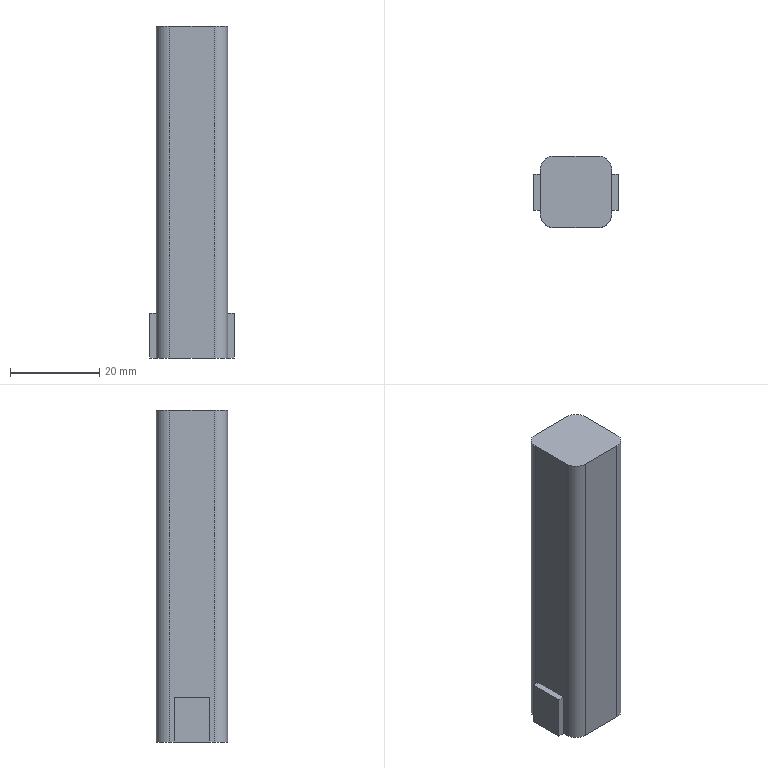Part | NX | features solid 2 | 1 solid | 18 faces | box 19 x 16 x 74.5 mm | volume 18736 mm3 | plane 14 | cylinder 4 | commonest cylinder face diameters 6 x4
STEP:
#1=CARTESIAN_POINT('',(2052.,45.,-68.));
#2=VERTEX_POINT('',#1);
#3=CARTESIAN_POINT('',(2052.,37.,-68.));
#4=VERTEX_POINT('',#3);
#5=CARTESIAN_POINT('',(2052.,41.,-68.));
#6=DIRECTION('',(0.,-1.,0.));
#7=VECTOR('',#6,1000.);
#8=LINE('',#5,#7);
#9=EDGE_CURVE('',#2,#4,#8,.T.);
#10=ORIENTED_EDGE('',*,*,#9,.T.);
#11=CARTESIAN_POINT('',(2052.,37.,-78.));
#12=VERTEX_POINT('',#11);
#13=CARTESIAN_POINT('',(2052.,37.,-63.));
#14=DIRECTION('',(0.,0.,-1.));
#15=VECTOR('',#14,1000.);
#16=LINE('',#13,#15);
#17=EDGE_CURVE('',#4,#12,#16,.T.);
#18=ORIENTED_EDGE('',*,*,#17,.T.);
#19=CARTESIAN_POINT('',(2052.,36.,-78.));
#20=VERTEX_POINT('',#19);
#21=CARTESIAN_POINT('',(2052.,41.,-78.));
#22=DIRECTION('',(0.,1.,0.));
#23=VECTOR('',#22,1000.);
#24=LINE('',#21,#23);
#25=EDGE_CURVE('',#20,#12,#24,.T.);
#26=ORIENTED_EDGE('',*,*,#25,.F.);
#27=CARTESIAN_POINT('',(2052.,36.,-3.5));
#28=VERTEX_POINT('',#27);
#29=CARTESIAN_POINT('',(2052.,36.,-63.));
#30=DIRECTION('',(0.,0.,1.));
#31=VECTOR('',#30,1000.);
#32=LINE('',#29,#31);
#33=EDGE_CURVE('',#20,#28,#32,.T.);
#34=ORIENTED_EDGE('',*,*,#33,.T.);
#35=CARTESIAN_POINT('',(2052.,46.,-3.5));
#36=VERTEX_POINT('',#35);
#37=CARTESIAN_POINT('',(2052.,41.,-3.5));
#38=DIRECTION('',(0.,1.,0.));
#39=VECTOR('',#38,1000.);
#40=LINE('',#37,#39);
#41=EDGE_CURVE('',#28,#36,#40,.T.);
#42=ORIENTED_EDGE('',*,*,#41,.T.);
#43=CARTESIAN_POINT('',(2052.,46.,-78.));
#44=VERTEX_POINT('',#43);
#45=CARTESIAN_POINT('',(2052.,46.,-63.));
#46=DIRECTION('',(0.,0.,-1.));
#47=VECTOR('',#46,1000.);
#48=LINE('',#45,#47);
#49=EDGE_CURVE('',#36,#44,#48,.T.);
#50=ORIENTED_EDGE('',*,*,#49,.T.);
#51=CARTESIAN_POINT('',(2052.,45.,-78.));
#52=VERTEX_POINT('',#51);
#53=CARTESIAN_POINT('',(2052.,41.,-78.));
#54=DIRECTION('',(0.,1.,0.));
#55=VECTOR('',#54,1000.);
#56=LINE('',#53,#55);
#57=EDGE_CURVE('',#52,#44,#56,.T.);
#58=ORIENTED_EDGE('',*,*,#57,.F.);
#59=CARTESIAN_POINT('',(2052.,45.,-63.));
#60=DIRECTION('',(0.,0.,1.));
#61=VECTOR('',#60,1000.);
#62=LINE('',#59,#61);
#63=EDGE_CURVE('',#52,#2,#62,.T.);
#64=ORIENTED_EDGE('',*,*,#63,.T.);
#65=EDGE_LOOP('',(#10,#18,#26,#34,#42,#50,#58,#64));
#66=FACE_BOUND('',#65,.T.);
#67=CARTESIAN_POINT('',(2052.,41.,-63.));
#68=DIRECTION('',(-1.,0.,0.));
#69=DIRECTION('',(0.,0.,-1.));
#70=AXIS2_PLACEMENT_3D('',#67,#68,#69);
#71=PLANE('',#70);
#72=ADVANCED_FACE('',(#66),#71,.T.);
#73=ORIENTED_EDGE('',*,*,#41,.F.);
#74=CARTESIAN_POINT('',(2055.,33.,-3.5));
#75=VERTEX_POINT('',#74);
#76=CARTESIAN_POINT('',(2055.,36.,-3.5));
#77=DIRECTION('',(0.,0.,1.));
#78=DIRECTION('',(1.,0.,0.));
#79=AXIS2_PLACEMENT_3D('',#76,#77,#78);
#80=CIRCLE('',#79,3.);
#81=EDGE_CURVE('',#28,#75,#80,.T.);
#82=ORIENTED_EDGE('',*,*,#81,.T.);
#83=CARTESIAN_POINT('',(2065.,33.,-3.5));
#84=VERTEX_POINT('',#83);
#85=CARTESIAN_POINT('',(2060.,33.,-3.5));
#86=DIRECTION('',(-1.,0.,0.));
#87=VECTOR('',#86,1000.);
#88=LINE('',#85,#87);
#89=EDGE_CURVE('',#84,#75,#88,.T.);
#90=ORIENTED_EDGE('',*,*,#89,.F.);
#91=CARTESIAN_POINT('',(2068.,36.,-3.5));
#92=VERTEX_POINT('',#91);
#93=CARTESIAN_POINT('',(2065.,36.,-3.5));
#94=DIRECTION('',(0.,0.,1.));
#95=DIRECTION('',(1.,0.,0.));
#96=AXIS2_PLACEMENT_3D('',#93,#94,#95);
#97=CIRCLE('',#96,3.);
#98=EDGE_CURVE('',#84,#92,#97,.T.);
#99=ORIENTED_EDGE('',*,*,#98,.T.);
#100=CARTESIAN_POINT('',(2068.,46.,-3.5));
#101=VERTEX_POINT('',#100);
#102=CARTESIAN_POINT('',(2068.,41.,-3.5));
#103=DIRECTION('',(0.,-1.,0.));
#104=VECTOR('',#103,1000.);
#105=LINE('',#102,#104);
#106=EDGE_CURVE('',#101,#92,#105,.T.);
#107=ORIENTED_EDGE('',*,*,#106,.F.);
#108=CARTESIAN_POINT('',(2065.,49.,-3.5));
#109=VERTEX_POINT('',#108);
#110=CARTESIAN_POINT('',(2065.,46.,-3.5));
#111=DIRECTION('',(0.,0.,1.));
#112=DIRECTION('',(1.,0.,0.));
#113=AXIS2_PLACEMENT_3D('',#110,#111,#112);
#114=CIRCLE('',#113,3.);
#115=EDGE_CURVE('',#101,#109,#114,.T.);
#116=ORIENTED_EDGE('',*,*,#115,.T.);
#117=CARTESIAN_POINT('',(2055.,49.,-3.5));
#118=VERTEX_POINT('',#117);
#119=CARTESIAN_POINT('',(2060.,49.,-3.5));
#120=DIRECTION('',(1.,0.,0.));
#121=VECTOR('',#120,1000.);
#122=LINE('',#119,#121);
#123=EDGE_CURVE('',#118,#109,#122,.T.);
#124=ORIENTED_EDGE('',*,*,#123,.F.);
#125=CARTESIAN_POINT('',(2055.,46.,-3.5));
#126=DIRECTION('',(0.,0.,1.));
#127=DIRECTION('',(1.,0.,0.));
#128=AXIS2_PLACEMENT_3D('',#125,#126,#127);
#129=CIRCLE('',#128,3.);
#130=EDGE_CURVE('',#118,#36,#129,.T.);
#131=ORIENTED_EDGE('',*,*,#130,.T.);
#132=EDGE_LOOP('',(#73,#82,#90,#99,#107,#116,#124,#131));
#133=FACE_BOUND('',#132,.T.);
#134=CARTESIAN_POINT('',(2060.,41.,-3.5));
#135=DIRECTION('',(0.,0.,1.));
#136=DIRECTION('',(-1.,0.,0.));
#137=AXIS2_PLACEMENT_3D('',#134,#135,#136);
#138=PLANE('',#137);
#139=ADVANCED_FACE('',(#133),#138,.T.);
#140=CARTESIAN_POINT('',(2055.,33.,-78.));
#141=VERTEX_POINT('',#140);
#142=CARTESIAN_POINT('',(2065.,33.,-78.));
#143=VERTEX_POINT('',#142);
#144=CARTESIAN_POINT('',(2060.,33.,-78.));
#145=DIRECTION('',(1.,0.,0.));
#146=VECTOR('',#145,1000.);
#147=LINE('',#144,#146);
#148=EDGE_CURVE('',#141,#143,#147,.T.);
#149=ORIENTED_EDGE('',*,*,#148,.T.);
#150=CARTESIAN_POINT('',(2065.,33.,-63.));
#151=DIRECTION('',(0.,0.,1.));
#152=VECTOR('',#151,1000.);
#153=LINE('',#150,#152);
#154=EDGE_CURVE('',#143,#84,#153,.T.);
#155=ORIENTED_EDGE('',*,*,#154,.T.);
#156=ORIENTED_EDGE('',*,*,#89,.T.);
#157=CARTESIAN_POINT('',(2055.,33.,-63.));
#158=DIRECTION('',(0.,0.,-1.));
#159=VECTOR('',#158,1000.);
#160=LINE('',#157,#159);
#161=EDGE_CURVE('',#75,#141,#160,.T.);
#162=ORIENTED_EDGE('',*,*,#161,.T.);
#163=EDGE_LOOP('',(#149,#155,#156,#162));
#164=FACE_BOUND('',#163,.T.);
#165=CARTESIAN_POINT('',(2060.,33.,-63.));
#166=DIRECTION('',(0.,-1.,0.));
#167=DIRECTION('',(0.,0.,1.));
#168=AXIS2_PLACEMENT_3D('',#165,#166,#167);
#169=PLANE('',#168);
#170=ADVANCED_FACE('',(#164),#169,.T.);
#171=CARTESIAN_POINT('',(2065.,49.,-78.));
#172=VERTEX_POINT('',#171);
#173=CARTESIAN_POINT('',(2055.,49.,-78.));
#174=VERTEX_POINT('',#173);
#175=CARTESIAN_POINT('',(2060.,49.,-78.));
#176=DIRECTION('',(-1.,0.,0.));
#177=VECTOR('',#176,1000.);
#178=LINE('',#175,#177);
#179=EDGE_CURVE('',#172,#174,#178,.T.);
#180=ORIENTED_EDGE('',*,*,#179,.T.);
#181=CARTESIAN_POINT('',(2055.,49.,-63.));
#182=DIRECTION('',(0.,0.,1.));
#183=VECTOR('',#182,1000.);
#184=LINE('',#181,#183);
#185=EDGE_CURVE('',#174,#118,#184,.T.);
#186=ORIENTED_EDGE('',*,*,#185,.T.);
#187=ORIENTED_EDGE('',*,*,#123,.T.);
#188=CARTESIAN_POINT('',(2065.,49.,-63.));
#189=DIRECTION('',(0.,0.,-1.));
#190=VECTOR('',#189,1000.);
#191=LINE('',#188,#190);
#192=EDGE_CURVE('',#109,#172,#191,.T.);
#193=ORIENTED_EDGE('',*,*,#192,.T.);
#194=EDGE_LOOP('',(#180,#186,#187,#193));
#195=FACE_BOUND('',#194,.T.);
#196=CARTESIAN_POINT('',(2060.,49.,-63.));
#197=DIRECTION('',(0.,1.,0.));
#198=DIRECTION('',(0.,0.,-1.));
#199=AXIS2_PLACEMENT_3D('',#196,#197,#198);
#200=PLANE('',#199);
#201=ADVANCED_FACE('',(#195),#200,.T.);
#202=CARTESIAN_POINT('',(2068.,45.,-78.));
#203=VERTEX_POINT('',#202);
#204=CARTESIAN_POINT('',(2068.,45.,-68.));
#205=VERTEX_POINT('',#204);
#206=CARTESIAN_POINT('',(2068.,45.,-63.));
#207=DIRECTION('',(0.,0.,1.));
#208=VECTOR('',#207,1000.);
#209=LINE('',#206,#208);
#210=EDGE_CURVE('',#203,#205,#209,.T.);
#211=ORIENTED_EDGE('',*,*,#210,.F.);
#212=CARTESIAN_POINT('',(2068.,46.,-78.));
#213=VERTEX_POINT('',#212);
#214=CARTESIAN_POINT('',(2068.,41.,-78.));
#215=DIRECTION('',(0.,-1.,0.));
#216=VECTOR('',#215,1000.);
#217=LINE('',#214,#216);
#218=EDGE_CURVE('',#213,#203,#217,.T.);
#219=ORIENTED_EDGE('',*,*,#218,.F.);
#220=CARTESIAN_POINT('',(2068.,46.,-63.));
#221=DIRECTION('',(0.,0.,1.));
#222=VECTOR('',#221,1000.);
#223=LINE('',#220,#222);
#224=EDGE_CURVE('',#213,#101,#223,.T.);
#225=ORIENTED_EDGE('',*,*,#224,.T.);
#226=ORIENTED_EDGE('',*,*,#106,.T.);
#227=CARTESIAN_POINT('',(2068.,36.,-78.));
#228=VERTEX_POINT('',#227);
#229=CARTESIAN_POINT('',(2068.,36.,-63.));
#230=DIRECTION('',(0.,0.,-1.));
#231=VECTOR('',#230,1000.);
#232=LINE('',#229,#231);
#233=EDGE_CURVE('',#92,#228,#232,.T.);
#234=ORIENTED_EDGE('',*,*,#233,.T.);
#235=CARTESIAN_POINT('',(2068.,37.,-78.));
#236=VERTEX_POINT('',#235);
#237=CARTESIAN_POINT('',(2068.,41.,-78.));
#238=DIRECTION('',(0.,-1.,0.));
#239=VECTOR('',#238,1000.);
#240=LINE('',#237,#239);
#241=EDGE_CURVE('',#236,#228,#240,.T.);
#242=ORIENTED_EDGE('',*,*,#241,.F.);
#243=CARTESIAN_POINT('',(2068.,37.,-68.));
#244=VERTEX_POINT('',#243);
#245=CARTESIAN_POINT('',(2068.,37.,-63.));
#246=DIRECTION('',(0.,0.,-1.));
#247=VECTOR('',#246,1000.);
#248=LINE('',#245,#247);
#249=EDGE_CURVE('',#244,#236,#248,.T.);
#250=ORIENTED_EDGE('',*,*,#249,.F.);
#251=CARTESIAN_POINT('',(2068.,41.,-68.));
#252=DIRECTION('',(0.,-1.,0.));
#253=VECTOR('',#252,1000.);
#254=LINE('',#251,#253);
#255=EDGE_CURVE('',#205,#244,#254,.T.);
#256=ORIENTED_EDGE('',*,*,#255,.F.);
#257=EDGE_LOOP('',(#211,#219,#225,#226,#234,#242,#250,#256));
#258=FACE_BOUND('',#257,.T.);
#259=CARTESIAN_POINT('',(2068.,41.,-63.));
#260=DIRECTION('',(1.,0.,0.));
#261=DIRECTION('',(0.,0.,1.));
#262=AXIS2_PLACEMENT_3D('',#259,#260,#261);
#263=PLANE('',#262);
#264=ADVANCED_FACE('',(#258),#263,.T.);
#265=CARTESIAN_POINT('',(2055.,36.,-78.));
#266=DIRECTION('',(0.,0.,-1.));
#267=DIRECTION('',(-1.,0.,0.));
#268=AXIS2_PLACEMENT_3D('',#265,#266,#267);
#269=CIRCLE('',#268,3.);
#270=EDGE_CURVE('',#141,#20,#269,.T.);
#271=ORIENTED_EDGE('',*,*,#270,.F.);
#272=ORIENTED_EDGE('',*,*,#161,.F.);
#273=ORIENTED_EDGE('',*,*,#81,.F.);
#274=ORIENTED_EDGE('',*,*,#33,.F.);
#275=EDGE_LOOP('',(#271,#272,#273,#274));
#276=FACE_BOUND('',#275,.T.);
#277=CARTESIAN_POINT('',(2055.,36.,-63.));
#278=DIRECTION('',(0.,0.,1.));
#279=DIRECTION('',(-1.,0.,0.));
#280=AXIS2_PLACEMENT_3D('',#277,#278,#279);
#281=CYLINDRICAL_SURFACE('',#280,3.);
#282=ADVANCED_FACE('',(#276),#281,.T.);
#283=CARTESIAN_POINT('',(2065.,36.,-78.));
#284=DIRECTION('',(0.,0.,-1.));
#285=DIRECTION('',(-1.,0.,0.));
#286=AXIS2_PLACEMENT_3D('',#283,#284,#285);
#287=CIRCLE('',#286,3.);
#288=EDGE_CURVE('',#228,#143,#287,.T.);
#289=ORIENTED_EDGE('',*,*,#288,.F.);
#290=ORIENTED_EDGE('',*,*,#233,.F.);
#291=ORIENTED_EDGE('',*,*,#98,.F.);
#292=ORIENTED_EDGE('',*,*,#154,.F.);
#293=EDGE_LOOP('',(#289,#290,#291,#292));
#294=FACE_BOUND('',#293,.T.);
#295=CARTESIAN_POINT('',(2065.,36.,-63.));
#296=DIRECTION('',(0.,0.,1.));
#297=DIRECTION('',(-1.,0.,0.));
#298=AXIS2_PLACEMENT_3D('',#295,#296,#297);
#299=CYLINDRICAL_SURFACE('',#298,3.);
#300=ADVANCED_FACE('',(#294),#299,.T.);
#301=CARTESIAN_POINT('',(2065.,46.,-78.));
#302=DIRECTION('',(0.,0.,-1.));
#303=DIRECTION('',(-1.,0.,0.));
#304=AXIS2_PLACEMENT_3D('',#301,#302,#303);
#305=CIRCLE('',#304,3.);
#306=EDGE_CURVE('',#172,#213,#305,.T.);
#307=ORIENTED_EDGE('',*,*,#306,.F.);
#308=ORIENTED_EDGE('',*,*,#192,.F.);
#309=ORIENTED_EDGE('',*,*,#115,.F.);
#310=ORIENTED_EDGE('',*,*,#224,.F.);
#311=EDGE_LOOP('',(#307,#308,#309,#310));
#312=FACE_BOUND('',#311,.T.);
#313=CARTESIAN_POINT('',(2065.,46.,-63.));
#314=DIRECTION('',(0.,0.,1.));
#315=DIRECTION('',(-1.,0.,0.));
#316=AXIS2_PLACEMENT_3D('',#313,#314,#315);
#317=CYLINDRICAL_SURFACE('',#316,3.);
#318=ADVANCED_FACE('',(#312),#317,.T.);
#319=CARTESIAN_POINT('',(2055.,46.,-78.));
#320=DIRECTION('',(0.,0.,-1.));
#321=DIRECTION('',(-1.,0.,0.));
#322=AXIS2_PLACEMENT_3D('',#319,#320,#321);
#323=CIRCLE('',#322,3.);
#324=EDGE_CURVE('',#44,#174,#323,.T.);
#325=ORIENTED_EDGE('',*,*,#324,.F.);
#326=ORIENTED_EDGE('',*,*,#49,.F.);
#327=ORIENTED_EDGE('',*,*,#130,.F.);
#328=ORIENTED_EDGE('',*,*,#185,.F.);
#329=EDGE_LOOP('',(#325,#326,#327,#328));
#330=FACE_BOUND('',#329,.T.);
#331=CARTESIAN_POINT('',(2055.,46.,-63.));
#332=DIRECTION('',(0.,0.,1.));
#333=DIRECTION('',(-1.,0.,0.));
#334=AXIS2_PLACEMENT_3D('',#331,#332,#333);
#335=CYLINDRICAL_SURFACE('',#334,3.);
#336=ADVANCED_FACE('',(#330),#335,.T.);
#337=ORIENTED_EDGE('',*,*,#306,.T.);
#338=ORIENTED_EDGE('',*,*,#218,.T.);
#339=CARTESIAN_POINT('',(2069.5,45.,-78.));
#340=VERTEX_POINT('',#339);
#341=CARTESIAN_POINT('',(2069.5,45.,-78.));
#342=DIRECTION('',(-1.,0.,0.));
#343=VECTOR('',#342,1000.);
#344=LINE('',#341,#343);
#345=EDGE_CURVE('',#340,#203,#344,.T.);
#346=ORIENTED_EDGE('',*,*,#345,.F.);
#347=CARTESIAN_POINT('',(2069.5,37.,-78.));
#348=VERTEX_POINT('',#347);
#349=CARTESIAN_POINT('',(2069.5,41.,-78.));
#350=DIRECTION('',(0.,-1.,0.));
#351=VECTOR('',#350,1000.);
#352=LINE('',#349,#351);
#353=EDGE_CURVE('',#340,#348,#352,.T.);
#354=ORIENTED_EDGE('',*,*,#353,.T.);
#355=CARTESIAN_POINT('',(2069.5,37.,-78.));
#356=DIRECTION('',(-1.,0.,0.));
#357=VECTOR('',#356,1000.);
#358=LINE('',#355,#357);
#359=EDGE_CURVE('',#348,#236,#358,.T.);
#360=ORIENTED_EDGE('',*,*,#359,.T.);
#361=ORIENTED_EDGE('',*,*,#241,.T.);
#362=ORIENTED_EDGE('',*,*,#288,.T.);
#363=ORIENTED_EDGE('',*,*,#148,.F.);
#364=ORIENTED_EDGE('',*,*,#270,.T.);
#365=ORIENTED_EDGE('',*,*,#25,.T.);
#366=CARTESIAN_POINT('',(2050.5,37.,-78.));
#367=VERTEX_POINT('',#366);
#368=CARTESIAN_POINT('',(2050.5,37.,-78.));
#369=DIRECTION('',(1.,0.,0.));
#370=VECTOR('',#369,1000.);
#371=LINE('',#368,#370);
#372=EDGE_CURVE('',#367,#12,#371,.T.);
#373=ORIENTED_EDGE('',*,*,#372,.F.);
#374=CARTESIAN_POINT('',(2050.5,45.,-78.));
#375=VERTEX_POINT('',#374);
#376=CARTESIAN_POINT('',(2050.5,41.,-78.));
#377=DIRECTION('',(0.,-1.,0.));
#378=VECTOR('',#377,1000.);
#379=LINE('',#376,#378);
#380=EDGE_CURVE('',#375,#367,#379,.T.);
#381=ORIENTED_EDGE('',*,*,#380,.F.);
#382=CARTESIAN_POINT('',(2050.5,45.,-78.));
#383=DIRECTION('',(1.,0.,0.));
#384=VECTOR('',#383,1000.);
#385=LINE('',#382,#384);
#386=EDGE_CURVE('',#375,#52,#385,.T.);
#387=ORIENTED_EDGE('',*,*,#386,.T.);
#388=ORIENTED_EDGE('',*,*,#57,.T.);
#389=ORIENTED_EDGE('',*,*,#324,.T.);
#390=ORIENTED_EDGE('',*,*,#179,.F.);
#391=EDGE_LOOP('',(#337,#338,#346,#354,#360,#361,#362,#363,#364,#365,#373,#381,#387,#388,#389,#390));
#392=FACE_BOUND('',#391,.T.);
#393=CARTESIAN_POINT('',(2060.,41.,-78.));
#394=DIRECTION('',(0.,0.,-1.));
#395=DIRECTION('',(1.,0.,0.));
#396=AXIS2_PLACEMENT_3D('',#393,#394,#395);
#397=PLANE('',#396);
#398=ADVANCED_FACE('',(#392),#397,.T.);
#399=CARTESIAN_POINT('',(2050.5,45.,-68.));
#400=VERTEX_POINT('',#399);
#401=CARTESIAN_POINT('',(2050.5,45.,-68.));
#402=DIRECTION('',(1.,0.,0.));
#403=VECTOR('',#402,1000.);
#404=LINE('',#401,#403);
#405=EDGE_CURVE('',#400,#2,#404,.T.);
#406=ORIENTED_EDGE('',*,*,#405,.T.);
#407=ORIENTED_EDGE('',*,*,#63,.F.);
#408=ORIENTED_EDGE('',*,*,#386,.F.);
#409=CARTESIAN_POINT('',(2050.5,45.,-63.));
#410=DIRECTION('',(0.,0.,1.));
#411=VECTOR('',#410,1000.);
#412=LINE('',#409,#411);
#413=EDGE_CURVE('',#375,#400,#412,.T.);
#414=ORIENTED_EDGE('',*,*,#413,.T.);
#415=EDGE_LOOP('',(#406,#407,#408,#414));
#416=FACE_BOUND('',#415,.T.);
#417=CARTESIAN_POINT('',(2050.5,45.,-63.));
#418=DIRECTION('',(0.,-1.,0.));
#419=DIRECTION('',(0.,0.,1.));
#420=AXIS2_PLACEMENT_3D('',#417,#418,#419);
#421=PLANE('',#420);
#422=ADVANCED_FACE('',(#416),#421,.F.);
#423=CARTESIAN_POINT('',(2050.5,37.,-68.));
#424=VERTEX_POINT('',#423);
#425=CARTESIAN_POINT('',(2050.5,37.,-68.));
#426=DIRECTION('',(-1.,0.,0.));
#427=VECTOR('',#426,1000.);
#428=LINE('',#425,#427);
#429=EDGE_CURVE('',#4,#424,#428,.T.);
#430=ORIENTED_EDGE('',*,*,#429,.T.);
#431=CARTESIAN_POINT('',(2050.5,37.,-63.));
#432=DIRECTION('',(0.,0.,-1.));
#433=VECTOR('',#432,1000.);
#434=LINE('',#431,#433);
#435=EDGE_CURVE('',#424,#367,#434,.T.);
#436=ORIENTED_EDGE('',*,*,#435,.T.);
#437=ORIENTED_EDGE('',*,*,#372,.T.);
#438=ORIENTED_EDGE('',*,*,#17,.F.);
#439=EDGE_LOOP('',(#430,#436,#437,#438));
#440=FACE_BOUND('',#439,.T.);
#441=CARTESIAN_POINT('',(2050.5,37.,-63.));
#442=DIRECTION('',(0.,1.,0.));
#443=DIRECTION('',(0.,0.,-1.));
#444=AXIS2_PLACEMENT_3D('',#441,#442,#443);
#445=PLANE('',#444);
#446=ADVANCED_FACE('',(#440),#445,.F.);
#447=ORIENTED_EDGE('',*,*,#413,.F.);
#448=ORIENTED_EDGE('',*,*,#380,.T.);
#449=ORIENTED_EDGE('',*,*,#435,.F.);
#450=CARTESIAN_POINT('',(2050.5,41.,-68.));
#451=DIRECTION('',(0.,-1.,0.));
#452=VECTOR('',#451,1000.);
#453=LINE('',#450,#452);
#454=EDGE_CURVE('',#400,#424,#453,.T.);
#455=ORIENTED_EDGE('',*,*,#454,.F.);
#456=EDGE_LOOP('',(#447,#448,#449,#455));
#457=FACE_BOUND('',#456,.T.);
#458=CARTESIAN_POINT('',(2050.5,41.,-63.));
#459=DIRECTION('',(-1.,0.,0.));
#460=DIRECTION('',(0.,0.,1.));
#461=AXIS2_PLACEMENT_3D('',#458,#459,#460);
#462=PLANE('',#461);
#463=ADVANCED_FACE('',(#457),#462,.T.);
#464=ORIENTED_EDGE('',*,*,#454,.T.);
#465=ORIENTED_EDGE('',*,*,#429,.F.);
#466=ORIENTED_EDGE('',*,*,#9,.F.);
#467=ORIENTED_EDGE('',*,*,#405,.F.);
#468=EDGE_LOOP('',(#464,#465,#466,#467));
#469=FACE_BOUND('',#468,.T.);
#470=CARTESIAN_POINT('',(2051.25,41.,-68.));
#471=DIRECTION('',(0.,0.,1.));
#472=DIRECTION('',(1.,0.,0.));
#473=AXIS2_PLACEMENT_3D('',#470,#471,#472);
#474=PLANE('',#473);
#475=ADVANCED_FACE('',(#469),#474,.T.);
#476=CARTESIAN_POINT('',(2069.5,45.,-68.));
#477=VERTEX_POINT('',#476);
#478=CARTESIAN_POINT('',(2069.5,45.,-68.));
#479=DIRECTION('',(-1.,0.,0.));
#480=VECTOR('',#479,1000.);
#481=LINE('',#478,#480);
#482=EDGE_CURVE('',#477,#205,#481,.T.);
#483=ORIENTED_EDGE('',*,*,#482,.F.);
#484=CARTESIAN_POINT('',(2069.5,45.,-63.));
#485=DIRECTION('',(0.,0.,1.));
#486=VECTOR('',#485,1000.);
#487=LINE('',#484,#486);
#488=EDGE_CURVE('',#340,#477,#487,.T.);
#489=ORIENTED_EDGE('',*,*,#488,.F.);
#490=ORIENTED_EDGE('',*,*,#345,.T.);
#491=ORIENTED_EDGE('',*,*,#210,.T.);
#492=EDGE_LOOP('',(#483,#489,#490,#491));
#493=FACE_BOUND('',#492,.T.);
#494=CARTESIAN_POINT('',(2069.5,45.,-63.));
#495=DIRECTION('',(0.,-1.,0.));
#496=DIRECTION('',(0.,0.,1.));
#497=AXIS2_PLACEMENT_3D('',#494,#495,#496);
#498=PLANE('',#497);
#499=ADVANCED_FACE('',(#493),#498,.F.);
#500=CARTESIAN_POINT('',(2069.5,37.,-68.));
#501=VERTEX_POINT('',#500);
#502=CARTESIAN_POINT('',(2069.5,37.,-68.));
#503=DIRECTION('',(1.,0.,0.));
#504=VECTOR('',#503,1000.);
#505=LINE('',#502,#504);
#506=EDGE_CURVE('',#244,#501,#505,.T.);
#507=ORIENTED_EDGE('',*,*,#506,.F.);
#508=ORIENTED_EDGE('',*,*,#249,.T.);
#509=ORIENTED_EDGE('',*,*,#359,.F.);
#510=CARTESIAN_POINT('',(2069.5,37.,-63.));
#511=DIRECTION('',(0.,0.,-1.));
#512=VECTOR('',#511,1000.);
#513=LINE('',#510,#512);
#514=EDGE_CURVE('',#501,#348,#513,.T.);
#515=ORIENTED_EDGE('',*,*,#514,.F.);
#516=EDGE_LOOP('',(#507,#508,#509,#515));
#517=FACE_BOUND('',#516,.T.);
#518=CARTESIAN_POINT('',(2069.5,37.,-63.));
#519=DIRECTION('',(0.,1.,0.));
#520=DIRECTION('',(0.,0.,-1.));
#521=AXIS2_PLACEMENT_3D('',#518,#519,#520);
#522=PLANE('',#521);
#523=ADVANCED_FACE('',(#517),#522,.F.);
#524=ORIENTED_EDGE('',*,*,#488,.T.);
#525=CARTESIAN_POINT('',(2069.5,41.,-68.));
#526=DIRECTION('',(0.,-1.,0.));
#527=VECTOR('',#526,1000.);
#528=LINE('',#525,#527);
#529=EDGE_CURVE('',#477,#501,#528,.T.);
#530=ORIENTED_EDGE('',*,*,#529,.T.);
#531=ORIENTED_EDGE('',*,*,#514,.T.);
#532=ORIENTED_EDGE('',*,*,#353,.F.);
#533=EDGE_LOOP('',(#524,#530,#531,#532));
#534=FACE_BOUND('',#533,.T.);
#535=CARTESIAN_POINT('',(2069.5,41.,-63.));
#536=DIRECTION('',(1.,0.,0.));
#537=DIRECTION('',(0.,0.,1.));
#538=AXIS2_PLACEMENT_3D('',#535,#536,#537);
#539=PLANE('',#538);
#540=ADVANCED_FACE('',(#534),#539,.T.);
#541=ORIENTED_EDGE('',*,*,#529,.F.);
#542=ORIENTED_EDGE('',*,*,#482,.T.);
#543=ORIENTED_EDGE('',*,*,#255,.T.);
#544=ORIENTED_EDGE('',*,*,#506,.T.);
#545=EDGE_LOOP('',(#541,#542,#543,#544));
#546=FACE_BOUND('',#545,.T.);
#547=CARTESIAN_POINT('',(2068.75,41.,-68.));
#548=DIRECTION('',(0.,0.,1.));
#549=DIRECTION('',(-1.,0.,0.));
#550=AXIS2_PLACEMENT_3D('',#547,#548,#549);
#551=PLANE('',#550);
#552=ADVANCED_FACE('',(#546),#551,.T.);
#553=CLOSED_SHELL('',(#72,#139,#170,#201,#264,#282,#300,#318,#336,#398,#422,#446,#463,#475,#499,#523,#540,#552));
#554=MANIFOLD_SOLID_BREP('',#553);
#555=(LENGTH_UNIT()NAMED_UNIT(*)SI_UNIT(.MILLI.,.METRE.));
#556=UNCERTAINTY_MEASURE_WITH_UNIT(LENGTH_MEASURE(0.00001),#555,'','');
#557=(NAMED_UNIT(*)PLANE_ANGLE_UNIT()SI_UNIT($,.RADIAN.));
#558=(NAMED_UNIT(*)SI_UNIT($,.STERADIAN.)SOLID_ANGLE_UNIT());
#559=(GEOMETRIC_REPRESENTATION_CONTEXT(3)GLOBAL_UNCERTAINTY_ASSIGNED_CONTEXT((#556))GLOBAL_UNIT_ASSIGNED_CONTEXT((#555,#557,#558))REPRESENTATION_CONTEXT('',''));
#560=ADVANCED_BREP_SHAPE_REPRESENTATION('',(#554),#559);